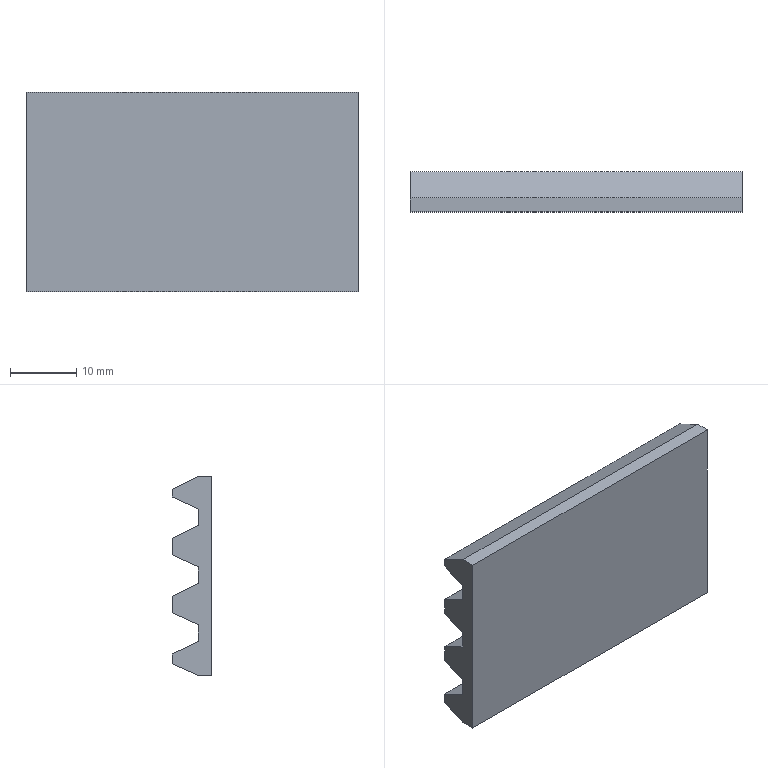Part | STEP file | Pressure plate 2 | 1 solid | 20 faces | box 50 x 6 x 30 mm | volume 6094 mm3 | plane 20
STEP:
#1=CARTESIAN_POINT('',(25.,6.,5.703));
#2=VERTEX_POINT('',#1);
#3=CARTESIAN_POINT('',(-25.,6.,5.703));
#4=VERTEX_POINT('',#3);
#5=CARTESIAN_POINT('',(0.,6.,5.703));
#6=DIRECTION('',(-1.,0.,0.));
#7=VECTOR('',#6,1000.);
#8=LINE('',#5,#7);
#9=EDGE_CURVE('',#2,#4,#8,.T.);
#10=ORIENTED_EDGE('',*,*,#9,.F.);
#11=CARTESIAN_POINT('',(25.,6.,3.172));
#12=VERTEX_POINT('',#11);
#13=CARTESIAN_POINT('',(25.,6.,-15.));
#14=DIRECTION('',(0.,0.,-1.));
#15=VECTOR('',#14,1000.);
#16=LINE('',#13,#15);
#17=EDGE_CURVE('',#2,#12,#16,.T.);
#18=ORIENTED_EDGE('',*,*,#17,.T.);
#19=CARTESIAN_POINT('',(-25.,6.,3.172));
#20=VERTEX_POINT('',#19);
#21=CARTESIAN_POINT('',(0.,6.,3.172));
#22=DIRECTION('',(1.,0.,0.));
#23=VECTOR('',#22,1000.);
#24=LINE('',#21,#23);
#25=EDGE_CURVE('',#20,#12,#24,.T.);
#26=ORIENTED_EDGE('',*,*,#25,.F.);
#27=CARTESIAN_POINT('',(-25.,6.,-15.));
#28=DIRECTION('',(0.,0.,1.));
#29=VECTOR('',#28,1000.);
#30=LINE('',#27,#29);
#31=EDGE_CURVE('',#20,#4,#30,.T.);
#32=ORIENTED_EDGE('',*,*,#31,.T.);
#33=EDGE_LOOP('',(#10,#18,#26,#32));
#34=FACE_OUTER_BOUND('',#33,.T.);
#35=CARTESIAN_POINT('',(0.,6.,0.));
#36=DIRECTION('',(0.,1.,0.));
#37=DIRECTION('',(0.,0.,1.));
#38=AXIS2_PLACEMENT_3D('',#35,#36,#37);
#39=PLANE('',#38);
#40=ADVANCED_FACE('',(#34),#39,.T.);
#41=CARTESIAN_POINT('',(25.,6.,-3.017));
#42=VERTEX_POINT('',#41);
#43=CARTESIAN_POINT('',(-25.,6.,-3.017));
#44=VERTEX_POINT('',#43);
#45=CARTESIAN_POINT('',(0.,6.,-3.017));
#46=DIRECTION('',(-1.,0.,0.));
#47=VECTOR('',#46,1000.);
#48=LINE('',#45,#47);
#49=EDGE_CURVE('',#42,#44,#48,.T.);
#50=ORIENTED_EDGE('',*,*,#49,.F.);
#51=CARTESIAN_POINT('',(25.,6.,-5.548));
#52=VERTEX_POINT('',#51);
#53=CARTESIAN_POINT('',(25.,6.,-15.));
#54=DIRECTION('',(0.,0.,-1.));
#55=VECTOR('',#54,1000.);
#56=LINE('',#53,#55);
#57=EDGE_CURVE('',#42,#52,#56,.T.);
#58=ORIENTED_EDGE('',*,*,#57,.T.);
#59=CARTESIAN_POINT('',(-25.,6.,-5.548));
#60=VERTEX_POINT('',#59);
#61=CARTESIAN_POINT('',(0.,6.,-5.548));
#62=DIRECTION('',(1.,0.,0.));
#63=VECTOR('',#62,1000.);
#64=LINE('',#61,#63);
#65=EDGE_CURVE('',#60,#52,#64,.T.);
#66=ORIENTED_EDGE('',*,*,#65,.F.);
#67=CARTESIAN_POINT('',(-25.,6.,-15.));
#68=DIRECTION('',(0.,0.,1.));
#69=VECTOR('',#68,1000.);
#70=LINE('',#67,#69);
#71=EDGE_CURVE('',#60,#44,#70,.T.);
#72=ORIENTED_EDGE('',*,*,#71,.T.);
#73=EDGE_LOOP('',(#50,#58,#66,#72));
#74=FACE_OUTER_BOUND('',#73,.T.);
#75=CARTESIAN_POINT('',(0.,6.,0.));
#76=DIRECTION('',(0.,1.,0.));
#77=DIRECTION('',(0.,0.,1.));
#78=AXIS2_PLACEMENT_3D('',#75,#76,#77);
#79=PLANE('',#78);
#80=ADVANCED_FACE('',(#74),#79,.T.);
#81=CARTESIAN_POINT('',(-25.,6.,-13.231));
#82=VERTEX_POINT('',#81);
#83=CARTESIAN_POINT('',(25.,6.,-13.231));
#84=VERTEX_POINT('',#83);
#85=CARTESIAN_POINT('',(0.,6.,-13.231));
#86=DIRECTION('',(1.,0.,0.));
#87=VECTOR('',#86,1000.);
#88=LINE('',#85,#87);
#89=EDGE_CURVE('',#82,#84,#88,.T.);
#90=ORIENTED_EDGE('',*,*,#89,.F.);
#91=CARTESIAN_POINT('',(-25.,6.,-11.737));
#92=VERTEX_POINT('',#91);
#93=CARTESIAN_POINT('',(-25.,6.,-15.));
#94=DIRECTION('',(0.,0.,1.));
#95=VECTOR('',#94,1000.);
#96=LINE('',#93,#95);
#97=EDGE_CURVE('',#82,#92,#96,.T.);
#98=ORIENTED_EDGE('',*,*,#97,.T.);
#99=CARTESIAN_POINT('',(25.,6.,-11.737));
#100=VERTEX_POINT('',#99);
#101=CARTESIAN_POINT('',(0.,6.,-11.737));
#102=DIRECTION('',(-1.,0.,0.));
#103=VECTOR('',#102,1000.);
#104=LINE('',#101,#103);
#105=EDGE_CURVE('',#100,#92,#104,.T.);
#106=ORIENTED_EDGE('',*,*,#105,.F.);
#107=CARTESIAN_POINT('',(25.,6.,-15.));
#108=DIRECTION('',(0.,0.,-1.));
#109=VECTOR('',#108,1000.);
#110=LINE('',#107,#109);
#111=EDGE_CURVE('',#100,#84,#110,.T.);
#112=ORIENTED_EDGE('',*,*,#111,.T.);
#113=EDGE_LOOP('',(#90,#98,#106,#112));
#114=FACE_OUTER_BOUND('',#113,.T.);
#115=CARTESIAN_POINT('',(0.,6.,0.));
#116=DIRECTION('',(0.,1.,0.));
#117=DIRECTION('',(0.,0.,1.));
#118=AXIS2_PLACEMENT_3D('',#115,#116,#117);
#119=PLANE('',#118);
#120=ADVANCED_FACE('',(#114),#119,.T.);
#121=CARTESIAN_POINT('',(25.,6.,13.082));
#122=VERTEX_POINT('',#121);
#123=CARTESIAN_POINT('',(25.,6.,11.892));
#124=VERTEX_POINT('',#123);
#125=CARTESIAN_POINT('',(25.,6.,-15.));
#126=DIRECTION('',(0.,0.,-1.));
#127=VECTOR('',#126,1000.);
#128=LINE('',#125,#127);
#129=EDGE_CURVE('',#122,#124,#128,.T.);
#130=ORIENTED_EDGE('',*,*,#129,.F.);
#131=CARTESIAN_POINT('',(25.,2.08,15.));
#132=VERTEX_POINT('',#131);
#133=CARTESIAN_POINT('',(25.,2.08,15.));
#134=DIRECTION('',(0.,0.8982,-0.4395));
#135=VECTOR('',#134,1000.);
#136=LINE('',#133,#135);
#137=EDGE_CURVE('',#132,#122,#136,.T.);
#138=ORIENTED_EDGE('',*,*,#137,.F.);
#139=CARTESIAN_POINT('',(25.,0.,15.));
#140=VERTEX_POINT('',#139);
#141=CARTESIAN_POINT('',(25.,6.,15.));
#142=DIRECTION('',(0.,-1.,0.));
#143=VECTOR('',#142,1000.);
#144=LINE('',#141,#143);
#145=EDGE_CURVE('',#132,#140,#144,.T.);
#146=ORIENTED_EDGE('',*,*,#145,.T.);
#147=CARTESIAN_POINT('',(25.,0.,-15.));
#148=VERTEX_POINT('',#147);
#149=CARTESIAN_POINT('',(25.,0.,-15.));
#150=DIRECTION('',(0.,0.,-1.));
#151=VECTOR('',#150,1000.);
#152=LINE('',#149,#151);
#153=EDGE_CURVE('',#140,#148,#152,.T.);
#154=ORIENTED_EDGE('',*,*,#153,.T.);
#155=CARTESIAN_POINT('',(25.,2.08,-15.));
#156=VERTEX_POINT('',#155);
#157=CARTESIAN_POINT('',(25.,6.,-15.));
#158=DIRECTION('',(0.,-1.,0.));
#159=VECTOR('',#158,1000.);
#160=LINE('',#157,#159);
#161=EDGE_CURVE('',#156,#148,#160,.T.);
#162=ORIENTED_EDGE('',*,*,#161,.F.);
#163=CARTESIAN_POINT('',(25.,2.08,-15.));
#164=DIRECTION('',(0.,-0.9115,-0.4114));
#165=VECTOR('',#164,1000.);
#166=LINE('',#163,#165);
#167=EDGE_CURVE('',#84,#156,#166,.T.);
#168=ORIENTED_EDGE('',*,*,#167,.F.);
#169=ORIENTED_EDGE('',*,*,#111,.F.);
#170=CARTESIAN_POINT('',(25.,2.08,-9.819));
#171=VERTEX_POINT('',#170);
#172=CARTESIAN_POINT('',(25.,2.08,-9.819));
#173=DIRECTION('',(0.,0.8982,-0.4395));
#174=VECTOR('',#173,1000.);
#175=LINE('',#172,#174);
#176=EDGE_CURVE('',#171,#100,#175,.T.);
#177=ORIENTED_EDGE('',*,*,#176,.F.);
#178=CARTESIAN_POINT('',(25.,2.08,-7.353));
#179=VERTEX_POINT('',#178);
#180=CARTESIAN_POINT('',(25.,2.08,-7.353));
#181=DIRECTION('',(0.,0.,-1.));
#182=VECTOR('',#181,1000.);
#183=LINE('',#180,#182);
#184=EDGE_CURVE('',#179,#171,#183,.T.);
#185=ORIENTED_EDGE('',*,*,#184,.F.);
#186=CARTESIAN_POINT('',(25.,6.,-5.548));
#187=DIRECTION('',(0.,-0.9084,-0.4182));
#188=VECTOR('',#187,1000.);
#189=LINE('',#186,#188);
#190=EDGE_CURVE('',#52,#179,#189,.T.);
#191=ORIENTED_EDGE('',*,*,#190,.F.);
#192=ORIENTED_EDGE('',*,*,#57,.F.);
#193=CARTESIAN_POINT('',(25.,2.08,-1.099));
#194=VERTEX_POINT('',#193);
#195=CARTESIAN_POINT('',(25.,2.08,-1.099));
#196=DIRECTION('',(0.,0.8982,-0.4395));
#197=VECTOR('',#196,1000.);
#198=LINE('',#195,#197);
#199=EDGE_CURVE('',#194,#42,#198,.T.);
#200=ORIENTED_EDGE('',*,*,#199,.F.);
#201=CARTESIAN_POINT('',(25.,2.08,1.367));
#202=VERTEX_POINT('',#201);
#203=CARTESIAN_POINT('',(25.,2.08,1.367));
#204=DIRECTION('',(0.,0.,-1.));
#205=VECTOR('',#204,1000.);
#206=LINE('',#203,#205);
#207=EDGE_CURVE('',#202,#194,#206,.T.);
#208=ORIENTED_EDGE('',*,*,#207,.F.);
#209=CARTESIAN_POINT('',(25.,6.,3.172));
#210=DIRECTION('',(0.,-0.9084,-0.4182));
#211=VECTOR('',#210,1000.);
#212=LINE('',#209,#211);
#213=EDGE_CURVE('',#12,#202,#212,.T.);
#214=ORIENTED_EDGE('',*,*,#213,.F.);
#215=ORIENTED_EDGE('',*,*,#17,.F.);
#216=CARTESIAN_POINT('',(25.,2.08,7.621));
#217=VERTEX_POINT('',#216);
#218=CARTESIAN_POINT('',(25.,2.08,7.621));
#219=DIRECTION('',(0.,0.8982,-0.4395));
#220=VECTOR('',#219,1000.);
#221=LINE('',#218,#220);
#222=EDGE_CURVE('',#217,#2,#221,.T.);
#223=ORIENTED_EDGE('',*,*,#222,.F.);
#224=CARTESIAN_POINT('',(25.,2.08,10.087));
#225=VERTEX_POINT('',#224);
#226=CARTESIAN_POINT('',(25.,2.08,10.087));
#227=DIRECTION('',(0.,0.,-1.));
#228=VECTOR('',#227,1000.);
#229=LINE('',#226,#228);
#230=EDGE_CURVE('',#225,#217,#229,.T.);
#231=ORIENTED_EDGE('',*,*,#230,.F.);
#232=CARTESIAN_POINT('',(25.,6.,11.892));
#233=DIRECTION('',(0.,-0.9084,-0.4182));
#234=VECTOR('',#233,1000.);
#235=LINE('',#232,#234);
#236=EDGE_CURVE('',#124,#225,#235,.T.);
#237=ORIENTED_EDGE('',*,*,#236,.F.);
#238=EDGE_LOOP('',(#130,#138,#146,#154,#162,#168,#169,#177,#185,#191,#192,#200,#208,#214,#215,#223,#231,#237));
#239=FACE_OUTER_BOUND('',#238,.T.);
#240=CARTESIAN_POINT('',(25.,6.,-15.));
#241=DIRECTION('',(-1.,0.,0.));
#242=DIRECTION('',(0.,0.,1.));
#243=AXIS2_PLACEMENT_3D('',#240,#241,#242);
#244=PLANE('',#243);
#245=ADVANCED_FACE('',(#239),#244,.F.);
#246=CARTESIAN_POINT('',(-25.,2.08,-15.));
#247=VERTEX_POINT('',#246);
#248=CARTESIAN_POINT('',(-25.,0.,-15.));
#249=VERTEX_POINT('',#248);
#250=CARTESIAN_POINT('',(-25.,6.,-15.));
#251=DIRECTION('',(0.,-1.,0.));
#252=VECTOR('',#251,1000.);
#253=LINE('',#250,#252);
#254=EDGE_CURVE('',#247,#249,#253,.T.);
#255=ORIENTED_EDGE('',*,*,#254,.F.);
#256=CARTESIAN_POINT('',(-36.,2.08,-15.));
#257=DIRECTION('',(1.,0.,0.));
#258=VECTOR('',#257,1000.);
#259=LINE('',#256,#258);
#260=EDGE_CURVE('',#247,#156,#259,.T.);
#261=ORIENTED_EDGE('',*,*,#260,.T.);
#262=ORIENTED_EDGE('',*,*,#161,.T.);
#263=CARTESIAN_POINT('',(-25.,0.,-15.));
#264=DIRECTION('',(-1.,0.,0.));
#265=VECTOR('',#264,1000.);
#266=LINE('',#263,#265);
#267=EDGE_CURVE('',#148,#249,#266,.T.);
#268=ORIENTED_EDGE('',*,*,#267,.T.);
#269=EDGE_LOOP('',(#255,#261,#262,#268));
#270=FACE_OUTER_BOUND('',#269,.T.);
#271=CARTESIAN_POINT('',(-25.,6.,-15.));
#272=DIRECTION('',(0.,0.,1.));
#273=DIRECTION('',(1.,0.,0.));
#274=AXIS2_PLACEMENT_3D('',#271,#272,#273);
#275=PLANE('',#274);
#276=ADVANCED_FACE('',(#270),#275,.F.);
#277=CARTESIAN_POINT('',(-25.,2.08,15.));
#278=VERTEX_POINT('',#277);
#279=CARTESIAN_POINT('',(-25.,0.,15.));
#280=VERTEX_POINT('',#279);
#281=CARTESIAN_POINT('',(-25.,6.,15.));
#282=DIRECTION('',(0.,-1.,0.));
#283=VECTOR('',#282,1000.);
#284=LINE('',#281,#283);
#285=EDGE_CURVE('',#278,#280,#284,.T.);
#286=ORIENTED_EDGE('',*,*,#285,.F.);
#287=CARTESIAN_POINT('',(-25.,6.,13.082));
#288=VERTEX_POINT('',#287);
#289=CARTESIAN_POINT('',(-25.,17.086,7.658));
#290=DIRECTION('',(0.,0.8982,-0.4395));
#291=VECTOR('',#290,1000.);
#292=LINE('',#289,#291);
#293=EDGE_CURVE('',#278,#288,#292,.T.);
#294=ORIENTED_EDGE('',*,*,#293,.T.);
#295=CARTESIAN_POINT('',(-25.,6.,11.892));
#296=VERTEX_POINT('',#295);
#297=CARTESIAN_POINT('',(-25.,6.,-15.));
#298=DIRECTION('',(0.,0.,1.));
#299=VECTOR('',#298,1000.);
#300=LINE('',#297,#299);
#301=EDGE_CURVE('',#296,#288,#300,.T.);
#302=ORIENTED_EDGE('',*,*,#301,.F.);
#303=CARTESIAN_POINT('',(-25.,2.08,10.087));
#304=VERTEX_POINT('',#303);
#305=CARTESIAN_POINT('',(-25.,-4.215,7.189));
#306=DIRECTION('',(0.,-0.9084,-0.4182));
#307=VECTOR('',#306,1000.);
#308=LINE('',#305,#307);
#309=EDGE_CURVE('',#296,#304,#308,.T.);
#310=ORIENTED_EDGE('',*,*,#309,.T.);
#311=CARTESIAN_POINT('',(-25.,2.08,7.621));
#312=VERTEX_POINT('',#311);
#313=CARTESIAN_POINT('',(-25.,2.08,-15.));
#314=DIRECTION('',(0.,0.,-1.));
#315=VECTOR('',#314,1000.);
#316=LINE('',#313,#315);
#317=EDGE_CURVE('',#304,#312,#316,.T.);
#318=ORIENTED_EDGE('',*,*,#317,.T.);
#319=CARTESIAN_POINT('',(-25.,14.173,1.704));
#320=DIRECTION('',(0.,0.8982,-0.4395));
#321=VECTOR('',#320,1000.);
#322=LINE('',#319,#321);
#323=EDGE_CURVE('',#312,#4,#322,.T.);
#324=ORIENTED_EDGE('',*,*,#323,.T.);
#325=ORIENTED_EDGE('',*,*,#31,.F.);
#326=CARTESIAN_POINT('',(-25.,2.08,1.367));
#327=VERTEX_POINT('',#326);
#328=CARTESIAN_POINT('',(-25.,-0.903,-0.005801));
#329=DIRECTION('',(0.,-0.9084,-0.4182));
#330=VECTOR('',#329,1000.);
#331=LINE('',#328,#330);
#332=EDGE_CURVE('',#20,#327,#331,.T.);
#333=ORIENTED_EDGE('',*,*,#332,.T.);
#334=CARTESIAN_POINT('',(-25.,2.08,-1.099));
#335=VERTEX_POINT('',#334);
#336=CARTESIAN_POINT('',(-25.,2.08,-15.));
#337=DIRECTION('',(0.,0.,-1.));
#338=VECTOR('',#337,1000.);
#339=LINE('',#336,#338);
#340=EDGE_CURVE('',#327,#335,#339,.T.);
#341=ORIENTED_EDGE('',*,*,#340,.T.);
#342=CARTESIAN_POINT('',(-25.,10.731,-5.331));
#343=DIRECTION('',(0.,0.8982,-0.4395));
#344=VECTOR('',#343,1000.);
#345=LINE('',#342,#344);
#346=EDGE_CURVE('',#335,#44,#345,.T.);
#347=ORIENTED_EDGE('',*,*,#346,.T.);
#348=ORIENTED_EDGE('',*,*,#71,.F.);
#349=CARTESIAN_POINT('',(-25.,2.08,-7.353));
#350=VERTEX_POINT('',#349);
#351=CARTESIAN_POINT('',(-25.,2.409,-7.201));
#352=DIRECTION('',(0.,-0.9084,-0.4182));
#353=VECTOR('',#352,1000.);
#354=LINE('',#351,#353);
#355=EDGE_CURVE('',#60,#350,#354,.T.);
#356=ORIENTED_EDGE('',*,*,#355,.T.);
#357=CARTESIAN_POINT('',(-25.,2.08,-9.819));
#358=VERTEX_POINT('',#357);
#359=CARTESIAN_POINT('',(-25.,2.08,-15.));
#360=DIRECTION('',(0.,0.,-1.));
#361=VECTOR('',#360,1000.);
#362=LINE('',#359,#361);
#363=EDGE_CURVE('',#350,#358,#362,.T.);
#364=ORIENTED_EDGE('',*,*,#363,.T.);
#365=CARTESIAN_POINT('',(-25.,7.288,-12.367));
#366=DIRECTION('',(0.,0.8982,-0.4395));
#367=VECTOR('',#366,1000.);
#368=LINE('',#365,#367);
#369=EDGE_CURVE('',#358,#92,#368,.T.);
#370=ORIENTED_EDGE('',*,*,#369,.T.);
#371=ORIENTED_EDGE('',*,*,#97,.F.);
#372=CARTESIAN_POINT('',(-25.,5.337,-13.53));
#373=DIRECTION('',(0.,-0.9115,-0.4114));
#374=VECTOR('',#373,1000.);
#375=LINE('',#372,#374);
#376=EDGE_CURVE('',#82,#247,#375,.T.);
#377=ORIENTED_EDGE('',*,*,#376,.T.);
#378=ORIENTED_EDGE('',*,*,#254,.T.);
#379=CARTESIAN_POINT('',(-25.,0.,-15.));
#380=DIRECTION('',(0.,0.,1.));
#381=VECTOR('',#380,1000.);
#382=LINE('',#379,#381);
#383=EDGE_CURVE('',#249,#280,#382,.T.);
#384=ORIENTED_EDGE('',*,*,#383,.T.);
#385=EDGE_LOOP('',(#286,#294,#302,#310,#318,#324,#325,#333,#341,#347,#348,#356,#364,#370,#371,#377,#378,#384));
#386=FACE_OUTER_BOUND('',#385,.T.);
#387=CARTESIAN_POINT('',(-25.,6.,-15.));
#388=DIRECTION('',(1.,0.,0.));
#389=DIRECTION('',(0.,0.,-1.));
#390=AXIS2_PLACEMENT_3D('',#387,#388,#389);
#391=PLANE('',#390);
#392=ADVANCED_FACE('',(#386),#391,.F.);
#393=ORIENTED_EDGE('',*,*,#145,.F.);
#394=CARTESIAN_POINT('',(-36.,2.08,15.));
#395=DIRECTION('',(1.,0.,0.));
#396=VECTOR('',#395,1000.);
#397=LINE('',#394,#396);
#398=EDGE_CURVE('',#278,#132,#397,.T.);
#399=ORIENTED_EDGE('',*,*,#398,.F.);
#400=ORIENTED_EDGE('',*,*,#285,.T.);
#401=CARTESIAN_POINT('',(-25.,0.,15.));
#402=DIRECTION('',(1.,0.,0.));
#403=VECTOR('',#402,1000.);
#404=LINE('',#401,#403);
#405=EDGE_CURVE('',#280,#140,#404,.T.);
#406=ORIENTED_EDGE('',*,*,#405,.T.);
#407=EDGE_LOOP('',(#393,#399,#400,#406));
#408=FACE_OUTER_BOUND('',#407,.T.);
#409=CARTESIAN_POINT('',(-25.,6.,15.));
#410=DIRECTION('',(0.,0.,-1.));
#411=DIRECTION('',(-1.,0.,0.));
#412=AXIS2_PLACEMENT_3D('',#409,#410,#411);
#413=PLANE('',#412);
#414=ADVANCED_FACE('',(#408),#413,.F.);
#415=CARTESIAN_POINT('',(0.,6.,13.082));
#416=DIRECTION('',(-1.,0.,0.));
#417=VECTOR('',#416,1000.);
#418=LINE('',#415,#417);
#419=EDGE_CURVE('',#122,#288,#418,.T.);
#420=ORIENTED_EDGE('',*,*,#419,.F.);
#421=ORIENTED_EDGE('',*,*,#129,.T.);
#422=CARTESIAN_POINT('',(0.,6.,11.892));
#423=DIRECTION('',(1.,0.,0.));
#424=VECTOR('',#423,1000.);
#425=LINE('',#422,#424);
#426=EDGE_CURVE('',#296,#124,#425,.T.);
#427=ORIENTED_EDGE('',*,*,#426,.F.);
#428=ORIENTED_EDGE('',*,*,#301,.T.);
#429=EDGE_LOOP('',(#420,#421,#427,#428));
#430=FACE_OUTER_BOUND('',#429,.T.);
#431=CARTESIAN_POINT('',(0.,6.,0.));
#432=DIRECTION('',(0.,1.,0.));
#433=DIRECTION('',(0.,0.,1.));
#434=AXIS2_PLACEMENT_3D('',#431,#432,#433);
#435=PLANE('',#434);
#436=ADVANCED_FACE('',(#430),#435,.T.);
#437=ORIENTED_EDGE('',*,*,#153,.F.);
#438=ORIENTED_EDGE('',*,*,#405,.F.);
#439=ORIENTED_EDGE('',*,*,#383,.F.);
#440=ORIENTED_EDGE('',*,*,#267,.F.);
#441=EDGE_LOOP('',(#437,#438,#439,#440));
#442=FACE_OUTER_BOUND('',#441,.T.);
#443=CARTESIAN_POINT('',(0.,0.,0.));
#444=DIRECTION('',(0.,1.,0.));
#445=DIRECTION('',(0.,0.,1.));
#446=AXIS2_PLACEMENT_3D('',#443,#444,#445);
#447=PLANE('',#446);
#448=ADVANCED_FACE('',(#442),#447,.F.);
#449=CARTESIAN_POINT('',(-36.,2.08,-7.353));
#450=DIRECTION('',(1.,0.,0.));
#451=VECTOR('',#450,1000.);
#452=LINE('',#449,#451);
#453=EDGE_CURVE('',#350,#179,#452,.T.);
#454=ORIENTED_EDGE('',*,*,#453,.T.);
#455=ORIENTED_EDGE('',*,*,#184,.T.);
#456=CARTESIAN_POINT('',(-36.,2.08,-9.819));
#457=DIRECTION('',(1.,0.,0.));
#458=VECTOR('',#457,1000.);
#459=LINE('',#456,#458);
#460=EDGE_CURVE('',#358,#171,#459,.T.);
#461=ORIENTED_EDGE('',*,*,#460,.F.);
#462=ORIENTED_EDGE('',*,*,#363,.F.);
#463=EDGE_LOOP('',(#454,#455,#461,#462));
#464=FACE_OUTER_BOUND('',#463,.T.);
#465=CARTESIAN_POINT('',(-36.,2.08,-7.353));
#466=DIRECTION('',(0.,-1.,0.));
#467=DIRECTION('',(0.,0.,-1.));
#468=AXIS2_PLACEMENT_3D('',#465,#466,#467);
#469=PLANE('',#468);
#470=ADVANCED_FACE('',(#464),#469,.F.);
#471=ORIENTED_EDGE('',*,*,#460,.T.);
#472=ORIENTED_EDGE('',*,*,#176,.T.);
#473=ORIENTED_EDGE('',*,*,#105,.T.);
#474=ORIENTED_EDGE('',*,*,#369,.F.);
#475=EDGE_LOOP('',(#471,#472,#473,#474));
#476=FACE_OUTER_BOUND('',#475,.T.);
#477=CARTESIAN_POINT('',(-36.,2.08,-9.819));
#478=DIRECTION('',(0.,-0.4395,-0.8982));
#479=DIRECTION('',(0.,0.8982,-0.4395));
#480=AXIS2_PLACEMENT_3D('',#477,#478,#479);
#481=PLANE('',#480);
#482=ADVANCED_FACE('',(#476),#481,.F.);
#483=ORIENTED_EDGE('',*,*,#65,.T.);
#484=ORIENTED_EDGE('',*,*,#190,.T.);
#485=ORIENTED_EDGE('',*,*,#453,.F.);
#486=ORIENTED_EDGE('',*,*,#355,.F.);
#487=EDGE_LOOP('',(#483,#484,#485,#486));
#488=FACE_OUTER_BOUND('',#487,.T.);
#489=CARTESIAN_POINT('',(-36.,6.,-5.548));
#490=DIRECTION('',(0.,-0.4182,0.9084));
#491=DIRECTION('',(0.,-0.9084,-0.4182));
#492=AXIS2_PLACEMENT_3D('',#489,#490,#491);
#493=PLANE('',#492);
#494=ADVANCED_FACE('',(#488),#493,.F.);
#495=ORIENTED_EDGE('',*,*,#89,.T.);
#496=ORIENTED_EDGE('',*,*,#167,.T.);
#497=ORIENTED_EDGE('',*,*,#260,.F.);
#498=ORIENTED_EDGE('',*,*,#376,.F.);
#499=EDGE_LOOP('',(#495,#496,#497,#498));
#500=FACE_OUTER_BOUND('',#499,.T.);
#501=CARTESIAN_POINT('',(-36.,2.08,-15.));
#502=DIRECTION('',(0.,-0.4114,0.9115));
#503=DIRECTION('',(0.,-0.9115,-0.4114));
#504=AXIS2_PLACEMENT_3D('',#501,#502,#503);
#505=PLANE('',#504);
#506=ADVANCED_FACE('',(#500),#505,.F.);
#507=CARTESIAN_POINT('',(-36.,2.08,1.367));
#508=DIRECTION('',(1.,0.,0.));
#509=VECTOR('',#508,1000.);
#510=LINE('',#507,#509);
#511=EDGE_CURVE('',#327,#202,#510,.T.);
#512=ORIENTED_EDGE('',*,*,#511,.T.);
#513=ORIENTED_EDGE('',*,*,#207,.T.);
#514=CARTESIAN_POINT('',(-36.,2.08,-1.099));
#515=DIRECTION('',(1.,0.,0.));
#516=VECTOR('',#515,1000.);
#517=LINE('',#514,#516);
#518=EDGE_CURVE('',#335,#194,#517,.T.);
#519=ORIENTED_EDGE('',*,*,#518,.F.);
#520=ORIENTED_EDGE('',*,*,#340,.F.);
#521=EDGE_LOOP('',(#512,#513,#519,#520));
#522=FACE_OUTER_BOUND('',#521,.T.);
#523=CARTESIAN_POINT('',(-36.,2.08,1.367));
#524=DIRECTION('',(0.,-1.,0.));
#525=DIRECTION('',(0.,0.,-1.));
#526=AXIS2_PLACEMENT_3D('',#523,#524,#525);
#527=PLANE('',#526);
#528=ADVANCED_FACE('',(#522),#527,.F.);
#529=ORIENTED_EDGE('',*,*,#518,.T.);
#530=ORIENTED_EDGE('',*,*,#199,.T.);
#531=ORIENTED_EDGE('',*,*,#49,.T.);
#532=ORIENTED_EDGE('',*,*,#346,.F.);
#533=EDGE_LOOP('',(#529,#530,#531,#532));
#534=FACE_OUTER_BOUND('',#533,.T.);
#535=CARTESIAN_POINT('',(-36.,2.08,-1.099));
#536=DIRECTION('',(0.,-0.4395,-0.8982));
#537=DIRECTION('',(0.,0.8982,-0.4395));
#538=AXIS2_PLACEMENT_3D('',#535,#536,#537);
#539=PLANE('',#538);
#540=ADVANCED_FACE('',(#534),#539,.F.);
#541=ORIENTED_EDGE('',*,*,#25,.T.);
#542=ORIENTED_EDGE('',*,*,#213,.T.);
#543=ORIENTED_EDGE('',*,*,#511,.F.);
#544=ORIENTED_EDGE('',*,*,#332,.F.);
#545=EDGE_LOOP('',(#541,#542,#543,#544));
#546=FACE_OUTER_BOUND('',#545,.T.);
#547=CARTESIAN_POINT('',(-36.,6.,3.172));
#548=DIRECTION('',(0.,-0.4182,0.9084));
#549=DIRECTION('',(0.,-0.9084,-0.4182));
#550=AXIS2_PLACEMENT_3D('',#547,#548,#549);
#551=PLANE('',#550);
#552=ADVANCED_FACE('',(#546),#551,.F.);
#553=CARTESIAN_POINT('',(-36.,2.08,10.087));
#554=DIRECTION('',(1.,0.,0.));
#555=VECTOR('',#554,1000.);
#556=LINE('',#553,#555);
#557=EDGE_CURVE('',#304,#225,#556,.T.);
#558=ORIENTED_EDGE('',*,*,#557,.T.);
#559=ORIENTED_EDGE('',*,*,#230,.T.);
#560=CARTESIAN_POINT('',(-36.,2.08,7.621));
#561=DIRECTION('',(1.,0.,0.));
#562=VECTOR('',#561,1000.);
#563=LINE('',#560,#562);
#564=EDGE_CURVE('',#312,#217,#563,.T.);
#565=ORIENTED_EDGE('',*,*,#564,.F.);
#566=ORIENTED_EDGE('',*,*,#317,.F.);
#567=EDGE_LOOP('',(#558,#559,#565,#566));
#568=FACE_OUTER_BOUND('',#567,.T.);
#569=CARTESIAN_POINT('',(-36.,2.08,10.087));
#570=DIRECTION('',(0.,-1.,0.));
#571=DIRECTION('',(0.,0.,-1.));
#572=AXIS2_PLACEMENT_3D('',#569,#570,#571);
#573=PLANE('',#572);
#574=ADVANCED_FACE('',(#568),#573,.F.);
#575=ORIENTED_EDGE('',*,*,#564,.T.);
#576=ORIENTED_EDGE('',*,*,#222,.T.);
#577=ORIENTED_EDGE('',*,*,#9,.T.);
#578=ORIENTED_EDGE('',*,*,#323,.F.);
#579=EDGE_LOOP('',(#575,#576,#577,#578));
#580=FACE_OUTER_BOUND('',#579,.T.);
#581=CARTESIAN_POINT('',(-36.,2.08,7.621));
#582=DIRECTION('',(0.,-0.4395,-0.8982));
#583=DIRECTION('',(0.,0.8982,-0.4395));
#584=AXIS2_PLACEMENT_3D('',#581,#582,#583);
#585=PLANE('',#584);
#586=ADVANCED_FACE('',(#580),#585,.F.);
#587=ORIENTED_EDGE('',*,*,#426,.T.);
#588=ORIENTED_EDGE('',*,*,#236,.T.);
#589=ORIENTED_EDGE('',*,*,#557,.F.);
#590=ORIENTED_EDGE('',*,*,#309,.F.);
#591=EDGE_LOOP('',(#587,#588,#589,#590));
#592=FACE_OUTER_BOUND('',#591,.T.);
#593=CARTESIAN_POINT('',(-36.,6.,11.892));
#594=DIRECTION('',(0.,-0.4182,0.9084));
#595=DIRECTION('',(0.,-0.9084,-0.4182));
#596=AXIS2_PLACEMENT_3D('',#593,#594,#595);
#597=PLANE('',#596);
#598=ADVANCED_FACE('',(#592),#597,.F.);
#599=ORIENTED_EDGE('',*,*,#398,.T.);
#600=ORIENTED_EDGE('',*,*,#137,.T.);
#601=ORIENTED_EDGE('',*,*,#419,.T.);
#602=ORIENTED_EDGE('',*,*,#293,.F.);
#603=EDGE_LOOP('',(#599,#600,#601,#602));
#604=FACE_OUTER_BOUND('',#603,.T.);
#605=CARTESIAN_POINT('',(-36.,2.08,15.));
#606=DIRECTION('',(0.,-0.4395,-0.8982));
#607=DIRECTION('',(0.,0.8982,-0.4395));
#608=AXIS2_PLACEMENT_3D('',#605,#606,#607);
#609=PLANE('',#608);
#610=ADVANCED_FACE('',(#604),#609,.F.);
#611=CLOSED_SHELL('',(#40,#80,#120,#245,#276,#392,#414,#436,#448,#470,#482,#494,#506,#528,#540,#552,#574,#586,#598,#610));
#612=MANIFOLD_SOLID_BREP('',#611);
#613=CARTESIAN_POINT('',(0.,0.,0.));
#614=DIRECTION('',(0.,0.,1.));
#615=DIRECTION('',(1.,0.,0.));
#616=AXIS2_PLACEMENT_3D('',#613,#614,#615);
#617=(LENGTH_UNIT()NAMED_UNIT(*)SI_UNIT(.MILLI.,.METRE.));
#618=UNCERTAINTY_MEASURE_WITH_UNIT(LENGTH_MEASURE(0.00001),#617,'','');
#619=(NAMED_UNIT(*)PLANE_ANGLE_UNIT()SI_UNIT($,.RADIAN.));
#620=(NAMED_UNIT(*)SI_UNIT($,.STERADIAN.)SOLID_ANGLE_UNIT());
#621=(GEOMETRIC_REPRESENTATION_CONTEXT(3)GLOBAL_UNCERTAINTY_ASSIGNED_CONTEXT((#618))GLOBAL_UNIT_ASSIGNED_CONTEXT((#617,#619,#620))REPRESENTATION_CONTEXT('',''));
#622=ADVANCED_BREP_SHAPE_REPRESENTATION('',(#612,#616),#621);